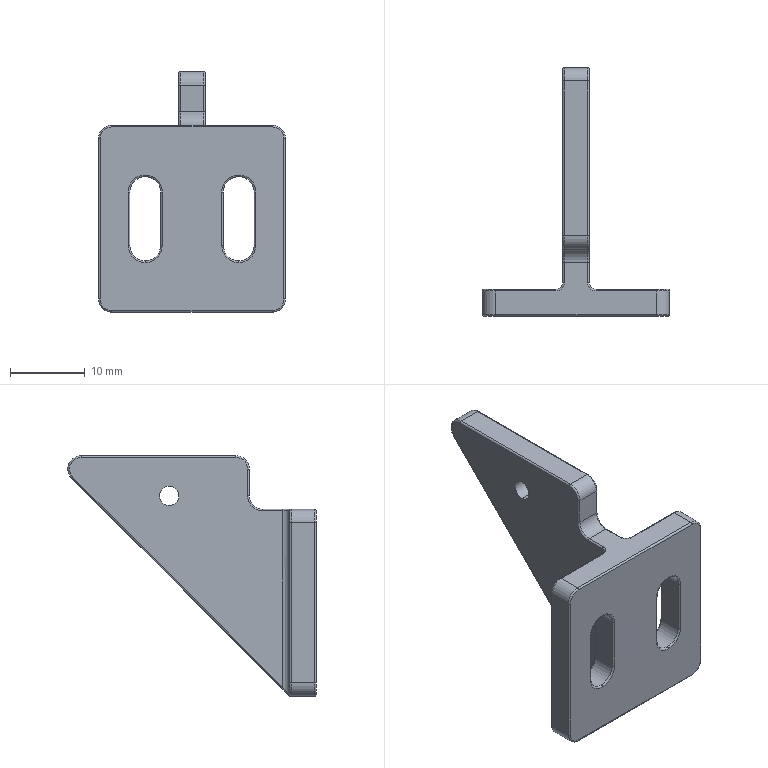Part | SolidWorks | features ICE 4, Fillet 3, Extrusion 1, Scale 1 | 1 solid | 94 faces | box 24.99 x 33.176 x 32.13 mm | volume 3593 mm3 | cylinder 44 | torus 30 | plane 16 | spline 2 | sphere 2 | commonest cylinder face diameters 0.446 x27 3.57 x7 4.106 x6 1.785 x2 2.6 x2